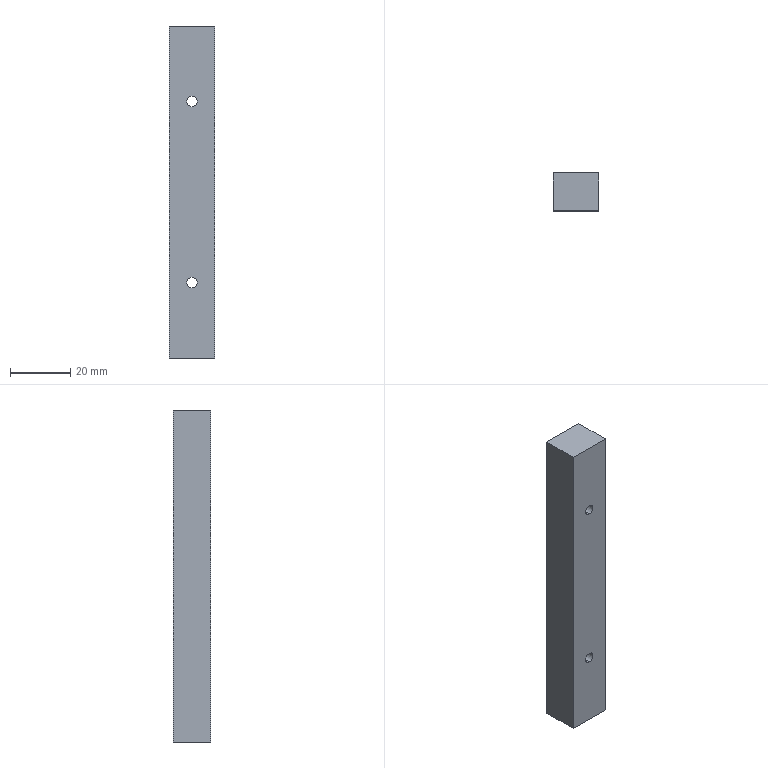Part | STEP file | Bag feed guide rail | 1 solid | 16 faces | box 15 x 12.5 x 110 mm | volume 20267 mm3 | cylinder 8 | plane 8 | commonest cylinder face diameters 3.4 x4 6 x4
STEP:
#1=CARTESIAN_POINT('',(0.,0.,0.));
#2=DIRECTION('',(0.,0.,1.));
#3=DIRECTION('',(1.,0.,0.));
#4=AXIS2_PLACEMENT_3D('',#1,#2,#3);
#5=CARTESIAN_POINT('',(0.,2.85,28.));
#6=VERTEX_POINT('',#5);
#7=CARTESIAN_POINT('',(0.,6.25,28.));
#8=VERTEX_POINT('',#7);
#9=CARTESIAN_POINT('',(0.,6.25,28.));
#10=DIRECTION('',(0.,1.,0.));
#11=VECTOR('',#10,1.);
#12=LINE('',#9,#11);
#13=CARTESIAN_POINT('',(0.,6.25,25.));
#14=DIRECTION('',(0.,1.,0.));
#15=DIRECTION('',(0.,0.,1.));
#16=AXIS2_PLACEMENT_3D('',#13,#14,#15);
#17=CYLINDRICAL_SURFACE('',#16,3.);
#18=CARTESIAN_POINT('',(6.283,0.));
#19=DIRECTION('',(0.,1.));
#20=VECTOR('',#19,1.);
#21=LINE('',#18,#20);
#22=(GEOMETRIC_REPRESENTATION_CONTEXT(2)PARAMETRIC_REPRESENTATION_CONTEXT()REPRESENTATION_CONTEXT('',''));
#23=DEFINITIONAL_REPRESENTATION('',(#21),#22);
#24=PCURVE('',#17,#23);
#25=CARTESIAN_POINT('',(0.,6.25,25.));
#26=DIRECTION('',(0.,1.,0.));
#27=DIRECTION('',(0.,0.,1.));
#28=AXIS2_PLACEMENT_3D('',#25,#26,#27);
#29=CYLINDRICAL_SURFACE('',#28,3.);
#30=CARTESIAN_POINT('',(0.,0.));
#31=DIRECTION('',(0.,1.));
#32=VECTOR('',#31,1.);
#33=LINE('',#30,#32);
#34=(GEOMETRIC_REPRESENTATION_CONTEXT(2)PARAMETRIC_REPRESENTATION_CONTEXT()REPRESENTATION_CONTEXT('',''));
#35=DEFINITIONAL_REPRESENTATION('',(#33),#34);
#36=PCURVE('',#29,#35);
#37=SURFACE_CURVE('',#12,(#24,#36),.PCURVE_S1.);
#38=EDGE_CURVE('',#6,#8,#37,.T.);
#39=ORIENTED_EDGE('',*,*,#38,.T.);
#40=CARTESIAN_POINT('',(0.,6.25,22.));
#41=VERTEX_POINT('',#40);
#42=CARTESIAN_POINT('',(0.,6.25,25.));
#43=DIRECTION('',(0.,1.,0.));
#44=DIRECTION('',(0.,0.,1.));
#45=AXIS2_PLACEMENT_3D('',#42,#43,#44);
#46=CIRCLE('',#45,3.);
#47=CARTESIAN_POINT('',(0.,0.));
#48=DIRECTION('',(1.,0.));
#49=VECTOR('',#48,1.);
#50=LINE('',#47,#49);
#51=(GEOMETRIC_REPRESENTATION_CONTEXT(2)PARAMETRIC_REPRESENTATION_CONTEXT()REPRESENTATION_CONTEXT('',''));
#52=DEFINITIONAL_REPRESENTATION('',(#50),#51);
#53=PCURVE('',#17,#52);
#54=CARTESIAN_POINT('',(-7.5,6.25,110.));
#55=DIRECTION('',(0.,-1.,0.));
#56=DIRECTION('',(0.,0.,-1.));
#57=AXIS2_PLACEMENT_3D('',#54,#55,#56);
#58=PLANE('',#57);
#59=CARTESIAN_POINT('',(82.,7.5));
#60=CARTESIAN_POINT('',(82.,12.696));
#61=CARTESIAN_POINT('',(86.5,10.098));
#62=CARTESIAN_POINT('',(91.,7.5));
#63=CARTESIAN_POINT('',(86.5,4.902));
#64=CARTESIAN_POINT('',(82.,2.304));
#65=CARTESIAN_POINT('',(82.,7.5));
#66=(BOUNDED_CURVE()B_SPLINE_CURVE(2,(#59,#60,#61,#62,#63,#64,#65),.UNSPECIFIED.,.T.,.F.)B_SPLINE_CURVE_WITH_KNOTS((1,2,2,2,2,1),(-2.094,0.,2.094,4.189,6.283,8.378),.UNSPECIFIED.)CURVE()GEOMETRIC_REPRESENTATION_ITEM()RATIONAL_B_SPLINE_CURVE((1.,0.5,1.,0.5,1.,0.5,1.))REPRESENTATION_ITEM(''));
#67=(GEOMETRIC_REPRESENTATION_CONTEXT(2)PARAMETRIC_REPRESENTATION_CONTEXT()REPRESENTATION_CONTEXT('',''));
#68=DEFINITIONAL_REPRESENTATION('',(#66),#67);
#69=PCURVE('',#58,#68);
#70=SURFACE_CURVE('',#46,(#53,#69),.PCURVE_S1.);
#71=EDGE_CURVE('',#41,#8,#70,.T.);
#72=ORIENTED_EDGE('',*,*,#71,.F.);
#73=CARTESIAN_POINT('',(0.,2.85,22.));
#74=VERTEX_POINT('',#73);
#75=CARTESIAN_POINT('',(0.,6.25,22.));
#76=DIRECTION('',(0.,1.,0.));
#77=VECTOR('',#76,1.);
#78=LINE('',#75,#77);
#79=CARTESIAN_POINT('',(3.142,0.));
#80=DIRECTION('',(0.,1.));
#81=VECTOR('',#80,1.);
#82=LINE('',#79,#81);
#83=(GEOMETRIC_REPRESENTATION_CONTEXT(2)PARAMETRIC_REPRESENTATION_CONTEXT()REPRESENTATION_CONTEXT('',''));
#84=DEFINITIONAL_REPRESENTATION('',(#82),#83);
#85=PCURVE('',#17,#84);
#86=CARTESIAN_POINT('',(3.142,0.));
#87=DIRECTION('',(0.,1.));
#88=VECTOR('',#87,1.);
#89=LINE('',#86,#88);
#90=(GEOMETRIC_REPRESENTATION_CONTEXT(2)PARAMETRIC_REPRESENTATION_CONTEXT()REPRESENTATION_CONTEXT('',''));
#91=DEFINITIONAL_REPRESENTATION('',(#89),#90);
#92=PCURVE('',#29,#91);
#93=SURFACE_CURVE('',#78,(#85,#92),.PCURVE_S1.);
#94=EDGE_CURVE('',#74,#41,#93,.T.);
#95=ORIENTED_EDGE('',*,*,#94,.F.);
#96=CARTESIAN_POINT('',(0.,2.85,25.));
#97=DIRECTION('',(0.,1.,0.));
#98=DIRECTION('',(0.,0.,1.));
#99=AXIS2_PLACEMENT_3D('',#96,#97,#98);
#100=CIRCLE('',#99,3.);
#101=CARTESIAN_POINT('',(0.,-3.4));
#102=DIRECTION('',(1.,0.));
#103=VECTOR('',#102,1.);
#104=LINE('',#101,#103);
#105=(GEOMETRIC_REPRESENTATION_CONTEXT(2)PARAMETRIC_REPRESENTATION_CONTEXT()REPRESENTATION_CONTEXT('',''));
#106=DEFINITIONAL_REPRESENTATION('',(#104),#105);
#107=PCURVE('',#17,#106);
#108=CARTESIAN_POINT('',(1.7,2.85,25.));
#109=DIRECTION('',(0.,-1.,0.));
#110=DIRECTION('',(0.,0.,-1.));
#111=AXIS2_PLACEMENT_3D('',#108,#109,#110);
#112=PLANE('',#111);
#113=CARTESIAN_POINT('',(-3.,-1.7));
#114=CARTESIAN_POINT('',(-3.,3.496));
#115=CARTESIAN_POINT('',(1.5,0.8981));
#116=CARTESIAN_POINT('',(6.,-1.7));
#117=CARTESIAN_POINT('',(1.5,-4.298));
#118=CARTESIAN_POINT('',(-3.,-6.896));
#119=CARTESIAN_POINT('',(-3.,-1.7));
#120=(BOUNDED_CURVE()B_SPLINE_CURVE(2,(#113,#114,#115,#116,#117,#118,#119),.UNSPECIFIED.,.T.,.F.)B_SPLINE_CURVE_WITH_KNOTS((1,2,2,2,2,1),(-2.094,0.,2.094,4.189,6.283,8.378),.UNSPECIFIED.)CURVE()GEOMETRIC_REPRESENTATION_ITEM()RATIONAL_B_SPLINE_CURVE((1.,0.5,1.,0.5,1.,0.5,1.))REPRESENTATION_ITEM(''));
#121=(GEOMETRIC_REPRESENTATION_CONTEXT(2)PARAMETRIC_REPRESENTATION_CONTEXT()REPRESENTATION_CONTEXT('',''));
#122=DEFINITIONAL_REPRESENTATION('',(#120),#121);
#123=PCURVE('',#112,#122);
#124=SURFACE_CURVE('',#100,(#107,#123),.PCURVE_S1.);
#125=EDGE_CURVE('',#74,#6,#124,.T.);
#126=ORIENTED_EDGE('',*,*,#125,.T.);
#127=EDGE_LOOP('',(#39,#72,#95,#126));
#128=FACE_BOUND('',#127,.F.);
#129=ADVANCED_FACE('',(#128),#17,.F.);
#130=CARTESIAN_POINT('',(0.,-6.25,26.7));
#131=VERTEX_POINT('',#130);
#132=CARTESIAN_POINT('',(0.,2.85,26.7));
#133=VERTEX_POINT('',#132);
#134=CARTESIAN_POINT('',(0.,6.25,26.7));
#135=DIRECTION('',(0.,1.,0.));
#136=VECTOR('',#135,1.);
#137=LINE('',#134,#136);
#138=CARTESIAN_POINT('',(0.,6.25,25.));
#139=DIRECTION('',(0.,1.,0.));
#140=DIRECTION('',(0.,0.,1.));
#141=AXIS2_PLACEMENT_3D('',#138,#139,#140);
#142=CYLINDRICAL_SURFACE('',#141,1.7);
#143=CARTESIAN_POINT('',(6.283,0.));
#144=DIRECTION('',(0.,1.));
#145=VECTOR('',#144,1.);
#146=LINE('',#143,#145);
#147=(GEOMETRIC_REPRESENTATION_CONTEXT(2)PARAMETRIC_REPRESENTATION_CONTEXT()REPRESENTATION_CONTEXT('',''));
#148=DEFINITIONAL_REPRESENTATION('',(#146),#147);
#149=PCURVE('',#142,#148);
#150=CARTESIAN_POINT('',(0.,6.25,25.));
#151=DIRECTION('',(0.,1.,0.));
#152=DIRECTION('',(0.,0.,1.));
#153=AXIS2_PLACEMENT_3D('',#150,#151,#152);
#154=CYLINDRICAL_SURFACE('',#153,1.7);
#155=CARTESIAN_POINT('',(0.,0.));
#156=DIRECTION('',(0.,1.));
#157=VECTOR('',#156,1.);
#158=LINE('',#155,#157);
#159=(GEOMETRIC_REPRESENTATION_CONTEXT(2)PARAMETRIC_REPRESENTATION_CONTEXT()REPRESENTATION_CONTEXT('',''));
#160=DEFINITIONAL_REPRESENTATION('',(#158),#159);
#161=PCURVE('',#154,#160);
#162=SURFACE_CURVE('',#137,(#149,#161),.PCURVE_S1.);
#163=EDGE_CURVE('',#131,#133,#162,.T.);
#164=ORIENTED_EDGE('',*,*,#163,.T.);
#165=CARTESIAN_POINT('',(0.,2.85,23.3));
#166=VERTEX_POINT('',#165);
#167=CARTESIAN_POINT('',(0.,2.85,25.));
#168=DIRECTION('',(0.,1.,0.));
#169=DIRECTION('',(0.,0.,1.));
#170=AXIS2_PLACEMENT_3D('',#167,#168,#169);
#171=CIRCLE('',#170,1.7);
#172=CARTESIAN_POINT('',(0.,-3.4));
#173=DIRECTION('',(1.,0.));
#174=VECTOR('',#173,1.);
#175=LINE('',#172,#174);
#176=(GEOMETRIC_REPRESENTATION_CONTEXT(2)PARAMETRIC_REPRESENTATION_CONTEXT()REPRESENTATION_CONTEXT('',''));
#177=DEFINITIONAL_REPRESENTATION('',(#175),#176);
#178=PCURVE('',#142,#177);
#179=CARTESIAN_POINT('',(-1.7,-1.7));
#180=CARTESIAN_POINT('',(-1.7,1.244));
#181=CARTESIAN_POINT('',(0.85,-0.2278));
#182=CARTESIAN_POINT('',(3.4,-1.7));
#183=CARTESIAN_POINT('',(0.85,-3.172));
#184=CARTESIAN_POINT('',(-1.7,-4.644));
#185=CARTESIAN_POINT('',(-1.7,-1.7));
#186=(BOUNDED_CURVE()B_SPLINE_CURVE(2,(#179,#180,#181,#182,#183,#184,#185),.UNSPECIFIED.,.T.,.F.)B_SPLINE_CURVE_WITH_KNOTS((1,2,2,2,2,1),(-2.094,0.,2.094,4.189,6.283,8.378),.UNSPECIFIED.)CURVE()GEOMETRIC_REPRESENTATION_ITEM()RATIONAL_B_SPLINE_CURVE((1.,0.5,1.,0.5,1.,0.5,1.))REPRESENTATION_ITEM(''));
#187=(GEOMETRIC_REPRESENTATION_CONTEXT(2)PARAMETRIC_REPRESENTATION_CONTEXT()REPRESENTATION_CONTEXT('',''));
#188=DEFINITIONAL_REPRESENTATION('',(#186),#187);
#189=PCURVE('',#112,#188);
#190=SURFACE_CURVE('',#171,(#178,#189),.PCURVE_S1.);
#191=EDGE_CURVE('',#166,#133,#190,.T.);
#192=ORIENTED_EDGE('',*,*,#191,.F.);
#193=CARTESIAN_POINT('',(0.,-6.25,23.3));
#194=VERTEX_POINT('',#193);
#195=CARTESIAN_POINT('',(0.,6.25,23.3));
#196=DIRECTION('',(0.,1.,0.));
#197=VECTOR('',#196,1.);
#198=LINE('',#195,#197);
#199=CARTESIAN_POINT('',(3.142,0.));
#200=DIRECTION('',(0.,1.));
#201=VECTOR('',#200,1.);
#202=LINE('',#199,#201);
#203=(GEOMETRIC_REPRESENTATION_CONTEXT(2)PARAMETRIC_REPRESENTATION_CONTEXT()REPRESENTATION_CONTEXT('',''));
#204=DEFINITIONAL_REPRESENTATION('',(#202),#203);
#205=PCURVE('',#142,#204);
#206=CARTESIAN_POINT('',(3.142,0.));
#207=DIRECTION('',(0.,1.));
#208=VECTOR('',#207,1.);
#209=LINE('',#206,#208);
#210=(GEOMETRIC_REPRESENTATION_CONTEXT(2)PARAMETRIC_REPRESENTATION_CONTEXT()REPRESENTATION_CONTEXT('',''));
#211=DEFINITIONAL_REPRESENTATION('',(#209),#210);
#212=PCURVE('',#154,#211);
#213=SURFACE_CURVE('',#198,(#205,#212),.PCURVE_S1.);
#214=EDGE_CURVE('',#194,#166,#213,.T.);
#215=ORIENTED_EDGE('',*,*,#214,.F.);
#216=CARTESIAN_POINT('',(0.,-6.25,25.));
#217=DIRECTION('',(0.,1.,0.));
#218=DIRECTION('',(0.,0.,1.));
#219=AXIS2_PLACEMENT_3D('',#216,#217,#218);
#220=CIRCLE('',#219,1.7);
#221=CARTESIAN_POINT('',(0.,-12.5));
#222=DIRECTION('',(1.,0.));
#223=VECTOR('',#222,1.);
#224=LINE('',#221,#223);
#225=(GEOMETRIC_REPRESENTATION_CONTEXT(2)PARAMETRIC_REPRESENTATION_CONTEXT()REPRESENTATION_CONTEXT('',''));
#226=DEFINITIONAL_REPRESENTATION('',(#224),#225);
#227=PCURVE('',#142,#226);
#228=CARTESIAN_POINT('',(-7.5,-6.25,110.));
#229=DIRECTION('',(0.,1.,0.));
#230=DIRECTION('',(0.,0.,1.));
#231=AXIS2_PLACEMENT_3D('',#228,#229,#230);
#232=PLANE('',#231);
#233=CARTESIAN_POINT('',(-85.,7.5));
#234=DIRECTION('',(1.,0.));
#235=AXIS2_PLACEMENT_2D('',#233,#234);
#236=CIRCLE('',#235,1.7);
#237=(GEOMETRIC_REPRESENTATION_CONTEXT(2)PARAMETRIC_REPRESENTATION_CONTEXT()REPRESENTATION_CONTEXT('',''));
#238=DEFINITIONAL_REPRESENTATION('',(#236),#237);
#239=PCURVE('',#232,#238);
#240=SURFACE_CURVE('',#220,(#227,#239),.PCURVE_S1.);
#241=EDGE_CURVE('',#194,#131,#240,.T.);
#242=ORIENTED_EDGE('',*,*,#241,.T.);
#243=EDGE_LOOP('',(#164,#192,#215,#242));
#244=FACE_BOUND('',#243,.F.);
#245=ADVANCED_FACE('',(#244),#142,.F.);
#246=CARTESIAN_POINT('',(0.,2.85,88.));
#247=VERTEX_POINT('',#246);
#248=CARTESIAN_POINT('',(0.,6.25,88.));
#249=VERTEX_POINT('',#248);
#250=CARTESIAN_POINT('',(0.,6.25,88.));
#251=DIRECTION('',(0.,1.,0.));
#252=VECTOR('',#251,1.);
#253=LINE('',#250,#252);
#254=CARTESIAN_POINT('',(0.,6.25,85.));
#255=DIRECTION('',(0.,1.,0.));
#256=DIRECTION('',(0.,0.,1.));
#257=AXIS2_PLACEMENT_3D('',#254,#255,#256);
#258=CYLINDRICAL_SURFACE('',#257,3.);
#259=CARTESIAN_POINT('',(6.283,0.));
#260=DIRECTION('',(0.,1.));
#261=VECTOR('',#260,1.);
#262=LINE('',#259,#261);
#263=(GEOMETRIC_REPRESENTATION_CONTEXT(2)PARAMETRIC_REPRESENTATION_CONTEXT()REPRESENTATION_CONTEXT('',''));
#264=DEFINITIONAL_REPRESENTATION('',(#262),#263);
#265=PCURVE('',#258,#264);
#266=CARTESIAN_POINT('',(0.,6.25,85.));
#267=DIRECTION('',(0.,1.,0.));
#268=DIRECTION('',(0.,0.,1.));
#269=AXIS2_PLACEMENT_3D('',#266,#267,#268);
#270=CYLINDRICAL_SURFACE('',#269,3.);
#271=CARTESIAN_POINT('',(0.,0.));
#272=DIRECTION('',(0.,1.));
#273=VECTOR('',#272,1.);
#274=LINE('',#271,#273);
#275=(GEOMETRIC_REPRESENTATION_CONTEXT(2)PARAMETRIC_REPRESENTATION_CONTEXT()REPRESENTATION_CONTEXT('',''));
#276=DEFINITIONAL_REPRESENTATION('',(#274),#275);
#277=PCURVE('',#270,#276);
#278=SURFACE_CURVE('',#253,(#265,#277),.PCURVE_S1.);
#279=EDGE_CURVE('',#247,#249,#278,.T.);
#280=ORIENTED_EDGE('',*,*,#279,.T.);
#281=CARTESIAN_POINT('',(0.,6.25,82.));
#282=VERTEX_POINT('',#281);
#283=CARTESIAN_POINT('',(0.,6.25,85.));
#284=DIRECTION('',(0.,1.,0.));
#285=DIRECTION('',(0.,0.,1.));
#286=AXIS2_PLACEMENT_3D('',#283,#284,#285);
#287=CIRCLE('',#286,3.);
#288=CARTESIAN_POINT('',(0.,0.));
#289=DIRECTION('',(1.,0.));
#290=VECTOR('',#289,1.);
#291=LINE('',#288,#290);
#292=(GEOMETRIC_REPRESENTATION_CONTEXT(2)PARAMETRIC_REPRESENTATION_CONTEXT()REPRESENTATION_CONTEXT('',''));
#293=DEFINITIONAL_REPRESENTATION('',(#291),#292);
#294=PCURVE('',#258,#293);
#295=CARTESIAN_POINT('',(22.,7.5));
#296=CARTESIAN_POINT('',(22.,12.696));
#297=CARTESIAN_POINT('',(26.5,10.098));
#298=CARTESIAN_POINT('',(31.,7.5));
#299=CARTESIAN_POINT('',(26.5,4.902));
#300=CARTESIAN_POINT('',(22.,2.304));
#301=CARTESIAN_POINT('',(22.,7.5));
#302=(BOUNDED_CURVE()B_SPLINE_CURVE(2,(#295,#296,#297,#298,#299,#300,#301),.UNSPECIFIED.,.T.,.F.)B_SPLINE_CURVE_WITH_KNOTS((1,2,2,2,2,1),(-2.094,0.,2.094,4.189,6.283,8.378),.UNSPECIFIED.)CURVE()GEOMETRIC_REPRESENTATION_ITEM()RATIONAL_B_SPLINE_CURVE((1.,0.5,1.,0.5,1.,0.5,1.))REPRESENTATION_ITEM(''));
#303=(GEOMETRIC_REPRESENTATION_CONTEXT(2)PARAMETRIC_REPRESENTATION_CONTEXT()REPRESENTATION_CONTEXT('',''));
#304=DEFINITIONAL_REPRESENTATION('',(#302),#303);
#305=PCURVE('',#58,#304);
#306=SURFACE_CURVE('',#287,(#294,#305),.PCURVE_S1.);
#307=EDGE_CURVE('',#282,#249,#306,.T.);
#308=ORIENTED_EDGE('',*,*,#307,.F.);
#309=CARTESIAN_POINT('',(0.,2.85,82.));
#310=VERTEX_POINT('',#309);
#311=CARTESIAN_POINT('',(0.,6.25,82.));
#312=DIRECTION('',(0.,1.,0.));
#313=VECTOR('',#312,1.);
#314=LINE('',#311,#313);
#315=CARTESIAN_POINT('',(3.142,0.));
#316=DIRECTION('',(0.,1.));
#317=VECTOR('',#316,1.);
#318=LINE('',#315,#317);
#319=(GEOMETRIC_REPRESENTATION_CONTEXT(2)PARAMETRIC_REPRESENTATION_CONTEXT()REPRESENTATION_CONTEXT('',''));
#320=DEFINITIONAL_REPRESENTATION('',(#318),#319);
#321=PCURVE('',#258,#320);
#322=CARTESIAN_POINT('',(3.142,0.));
#323=DIRECTION('',(0.,1.));
#324=VECTOR('',#323,1.);
#325=LINE('',#322,#324);
#326=(GEOMETRIC_REPRESENTATION_CONTEXT(2)PARAMETRIC_REPRESENTATION_CONTEXT()REPRESENTATION_CONTEXT('',''));
#327=DEFINITIONAL_REPRESENTATION('',(#325),#326);
#328=PCURVE('',#270,#327);
#329=SURFACE_CURVE('',#314,(#321,#328),.PCURVE_S1.);
#330=EDGE_CURVE('',#310,#282,#329,.T.);
#331=ORIENTED_EDGE('',*,*,#330,.F.);
#332=CARTESIAN_POINT('',(0.,2.85,85.));
#333=DIRECTION('',(0.,1.,0.));
#334=DIRECTION('',(0.,0.,1.));
#335=AXIS2_PLACEMENT_3D('',#332,#333,#334);
#336=CIRCLE('',#335,3.);
#337=CARTESIAN_POINT('',(0.,-3.4));
#338=DIRECTION('',(1.,0.));
#339=VECTOR('',#338,1.);
#340=LINE('',#337,#339);
#341=(GEOMETRIC_REPRESENTATION_CONTEXT(2)PARAMETRIC_REPRESENTATION_CONTEXT()REPRESENTATION_CONTEXT('',''));
#342=DEFINITIONAL_REPRESENTATION('',(#340),#341);
#343=PCURVE('',#258,#342);
#344=CARTESIAN_POINT('',(1.7,2.85,85.));
#345=DIRECTION('',(0.,-1.,0.));
#346=DIRECTION('',(0.,0.,-1.));
#347=AXIS2_PLACEMENT_3D('',#344,#345,#346);
#348=PLANE('',#347);
#349=CARTESIAN_POINT('',(-3.,-1.7));
#350=CARTESIAN_POINT('',(-3.,3.496));
#351=CARTESIAN_POINT('',(1.5,0.8981));
#352=CARTESIAN_POINT('',(6.,-1.7));
#353=CARTESIAN_POINT('',(1.5,-4.298));
#354=CARTESIAN_POINT('',(-3.,-6.896));
#355=CARTESIAN_POINT('',(-3.,-1.7));
#356=(BOUNDED_CURVE()B_SPLINE_CURVE(2,(#349,#350,#351,#352,#353,#354,#355),.UNSPECIFIED.,.T.,.F.)B_SPLINE_CURVE_WITH_KNOTS((1,2,2,2,2,1),(-2.094,0.,2.094,4.189,6.283,8.378),.UNSPECIFIED.)CURVE()GEOMETRIC_REPRESENTATION_ITEM()RATIONAL_B_SPLINE_CURVE((1.,0.5,1.,0.5,1.,0.5,1.))REPRESENTATION_ITEM(''));
#357=(GEOMETRIC_REPRESENTATION_CONTEXT(2)PARAMETRIC_REPRESENTATION_CONTEXT()REPRESENTATION_CONTEXT('',''));
#358=DEFINITIONAL_REPRESENTATION('',(#356),#357);
#359=PCURVE('',#348,#358);
#360=SURFACE_CURVE('',#336,(#343,#359),.PCURVE_S1.);
#361=EDGE_CURVE('',#310,#247,#360,.T.);
#362=ORIENTED_EDGE('',*,*,#361,.T.);
#363=EDGE_LOOP('',(#280,#308,#331,#362));
#364=FACE_BOUND('',#363,.F.);
#365=ADVANCED_FACE('',(#364),#258,.F.);
#366=CARTESIAN_POINT('',(0.,-6.25,86.7));
#367=VERTEX_POINT('',#366);
#368=CARTESIAN_POINT('',(0.,2.85,86.7));
#369=VERTEX_POINT('',#368);
#370=CARTESIAN_POINT('',(0.,6.25,86.7));
#371=DIRECTION('',(0.,1.,0.));
#372=VECTOR('',#371,1.);
#373=LINE('',#370,#372);
#374=CARTESIAN_POINT('',(0.,6.25,85.));
#375=DIRECTION('',(0.,1.,0.));
#376=DIRECTION('',(0.,0.,1.));
#377=AXIS2_PLACEMENT_3D('',#374,#375,#376);
#378=CYLINDRICAL_SURFACE('',#377,1.7);
#379=CARTESIAN_POINT('',(6.283,0.));
#380=DIRECTION('',(0.,1.));
#381=VECTOR('',#380,1.);
#382=LINE('',#379,#381);
#383=(GEOMETRIC_REPRESENTATION_CONTEXT(2)PARAMETRIC_REPRESENTATION_CONTEXT()REPRESENTATION_CONTEXT('',''));
#384=DEFINITIONAL_REPRESENTATION('',(#382),#383);
#385=PCURVE('',#378,#384);
#386=CARTESIAN_POINT('',(0.,6.25,85.));
#387=DIRECTION('',(0.,1.,0.));
#388=DIRECTION('',(0.,0.,1.));
#389=AXIS2_PLACEMENT_3D('',#386,#387,#388);
#390=CYLINDRICAL_SURFACE('',#389,1.7);
#391=CARTESIAN_POINT('',(0.,0.));
#392=DIRECTION('',(0.,1.));
#393=VECTOR('',#392,1.);
#394=LINE('',#391,#393);
#395=(GEOMETRIC_REPRESENTATION_CONTEXT(2)PARAMETRIC_REPRESENTATION_CONTEXT()REPRESENTATION_CONTEXT('',''));
#396=DEFINITIONAL_REPRESENTATION('',(#394),#395);
#397=PCURVE('',#390,#396);
#398=SURFACE_CURVE('',#373,(#385,#397),.PCURVE_S1.);
#399=EDGE_CURVE('',#367,#369,#398,.T.);
#400=ORIENTED_EDGE('',*,*,#399,.T.);
#401=CARTESIAN_POINT('',(0.,2.85,83.3));
#402=VERTEX_POINT('',#401);
#403=CARTESIAN_POINT('',(0.,2.85,85.));
#404=DIRECTION('',(0.,1.,0.));
#405=DIRECTION('',(0.,0.,1.));
#406=AXIS2_PLACEMENT_3D('',#403,#404,#405);
#407=CIRCLE('',#406,1.7);
#408=CARTESIAN_POINT('',(0.,-3.4));
#409=DIRECTION('',(1.,0.));
#410=VECTOR('',#409,1.);
#411=LINE('',#408,#410);
#412=(GEOMETRIC_REPRESENTATION_CONTEXT(2)PARAMETRIC_REPRESENTATION_CONTEXT()REPRESENTATION_CONTEXT('',''));
#413=DEFINITIONAL_REPRESENTATION('',(#411),#412);
#414=PCURVE('',#378,#413);
#415=CARTESIAN_POINT('',(-1.7,-1.7));
#416=CARTESIAN_POINT('',(-1.7,1.244));
#417=CARTESIAN_POINT('',(0.85,-0.2278));
#418=CARTESIAN_POINT('',(3.4,-1.7));
#419=CARTESIAN_POINT('',(0.85,-3.172));
#420=CARTESIAN_POINT('',(-1.7,-4.644));
#421=CARTESIAN_POINT('',(-1.7,-1.7));
#422=(BOUNDED_CURVE()B_SPLINE_CURVE(2,(#415,#416,#417,#418,#419,#420,#421),.UNSPECIFIED.,.T.,.F.)B_SPLINE_CURVE_WITH_KNOTS((1,2,2,2,2,1),(-2.094,0.,2.094,4.189,6.283,8.378),.UNSPECIFIED.)CURVE()GEOMETRIC_REPRESENTATION_ITEM()RATIONAL_B_SPLINE_CURVE((1.,0.5,1.,0.5,1.,0.5,1.))REPRESENTATION_ITEM(''));
#423=(GEOMETRIC_REPRESENTATION_CONTEXT(2)PARAMETRIC_REPRESENTATION_CONTEXT()REPRESENTATION_CONTEXT('',''));
#424=DEFINITIONAL_REPRESENTATION('',(#422),#423);
#425=PCURVE('',#348,#424);
#426=SURFACE_CURVE('',#407,(#414,#425),.PCURVE_S1.);
#427=EDGE_CURVE('',#402,#369,#426,.T.);
#428=ORIENTED_EDGE('',*,*,#427,.F.);
#429=CARTESIAN_POINT('',(0.,-6.25,83.3));
#430=VERTEX_POINT('',#429);
#431=CARTESIAN_POINT('',(0.,6.25,83.3));
#432=DIRECTION('',(0.,1.,0.));
#433=VECTOR('',#432,1.);
#434=LINE('',#431,#433);
#435=CARTESIAN_POINT('',(3.142,0.));
#436=DIRECTION('',(0.,1.));
#437=VECTOR('',#436,1.);
#438=LINE('',#435,#437);
#439=(GEOMETRIC_REPRESENTATION_CONTEXT(2)PARAMETRIC_REPRESENTATION_CONTEXT()REPRESENTATION_CONTEXT('',''));
#440=DEFINITIONAL_REPRESENTATION('',(#438),#439);
#441=PCURVE('',#378,#440);
#442=CARTESIAN_POINT('',(3.142,0.));
#443=DIRECTION('',(0.,1.));
#444=VECTOR('',#443,1.);
#445=LINE('',#442,#444);
#446=(GEOMETRIC_REPRESENTATION_CONTEXT(2)PARAMETRIC_REPRESENTATION_CONTEXT()REPRESENTATION_CONTEXT('',''));
#447=DEFINITIONAL_REPRESENTATION('',(#445),#446);
#448=PCURVE('',#390,#447);
#449=SURFACE_CURVE('',#434,(#441,#448),.PCURVE_S1.);
#450=EDGE_CURVE('',#430,#402,#449,.T.);
#451=ORIENTED_EDGE('',*,*,#450,.F.);
#452=CARTESIAN_POINT('',(0.,-6.25,85.));
#453=DIRECTION('',(0.,1.,0.));
#454=DIRECTION('',(0.,0.,1.));
#455=AXIS2_PLACEMENT_3D('',#452,#453,#454);
#456=CIRCLE('',#455,1.7);
#457=CARTESIAN_POINT('',(0.,-12.5));
#458=DIRECTION('',(1.,0.));
#459=VECTOR('',#458,1.);
#460=LINE('',#457,#459);
#461=(GEOMETRIC_REPRESENTATION_CONTEXT(2)PARAMETRIC_REPRESENTATION_CONTEXT()REPRESENTATION_CONTEXT('',''));
#462=DEFINITIONAL_REPRESENTATION('',(#460),#461);
#463=PCURVE('',#378,#462);
#464=CARTESIAN_POINT('',(-25.,7.5));
#465=DIRECTION('',(1.,0.));
#466=AXIS2_PLACEMENT_2D('',#464,#465);
#467=CIRCLE('',#466,1.7);
#468=(GEOMETRIC_REPRESENTATION_CONTEXT(2)PARAMETRIC_REPRESENTATION_CONTEXT()REPRESENTATION_CONTEXT('',''));
#469=DEFINITIONAL_REPRESENTATION('',(#467),#468);
#470=PCURVE('',#232,#469);
#471=SURFACE_CURVE('',#456,(#463,#470),.PCURVE_S1.);
#472=EDGE_CURVE('',#430,#367,#471,.T.);
#473=ORIENTED_EDGE('',*,*,#472,.T.);
#474=EDGE_LOOP('',(#400,#428,#451,#473));
#475=FACE_BOUND('',#474,.F.);
#476=ADVANCED_FACE('',(#475),#378,.F.);
#477=CARTESIAN_POINT('',(7.5,-6.25,0.));
#478=VERTEX_POINT('',#477);
#479=CARTESIAN_POINT('',(7.5,6.25,0.));
#480=VERTEX_POINT('',#479);
#481=CARTESIAN_POINT('',(7.5,-6.25,0.));
#482=DIRECTION('',(0.,1.,0.));
#483=VECTOR('',#482,1.);
#484=LINE('',#481,#483);
#485=CARTESIAN_POINT('',(7.5,-6.25,110.));
#486=DIRECTION('',(-1.,0.,0.));
#487=DIRECTION('',(0.,0.,1.));
#488=AXIS2_PLACEMENT_3D('',#485,#486,#487);
#489=PLANE('',#488);
#490=CARTESIAN_POINT('',(-110.,0.));
#491=DIRECTION('',(0.,1.));
#492=VECTOR('',#491,1.);
#493=LINE('',#490,#492);
#494=(GEOMETRIC_REPRESENTATION_CONTEXT(2)PARAMETRIC_REPRESENTATION_CONTEXT()REPRESENTATION_CONTEXT('',''));
#495=DEFINITIONAL_REPRESENTATION('',(#493),#494);
#496=PCURVE('',#489,#495);
#497=CARTESIAN_POINT('',(0.,0.,0.));
#498=DIRECTION('',(0.,0.,-1.));
#499=DIRECTION('',(-1.,0.,0.));
#500=AXIS2_PLACEMENT_3D('',#497,#498,#499);
#501=PLANE('',#500);
#502=CARTESIAN_POINT('',(-7.5,-6.25));
#503=DIRECTION('',(0.,1.));
#504=VECTOR('',#503,1.);
#505=LINE('',#502,#504);
#506=(GEOMETRIC_REPRESENTATION_CONTEXT(2)PARAMETRIC_REPRESENTATION_CONTEXT()REPRESENTATION_CONTEXT('',''));
#507=DEFINITIONAL_REPRESENTATION('',(#505),#506);
#508=PCURVE('',#501,#507);
#509=SURFACE_CURVE('',#484,(#496,#508),.PCURVE_S1.);
#510=EDGE_CURVE('',#478,#480,#509,.T.);
#511=ORIENTED_EDGE('',*,*,#510,.T.);
#512=CARTESIAN_POINT('',(7.5,6.25,110.));
#513=VERTEX_POINT('',#512);
#514=CARTESIAN_POINT('',(7.5,6.25,110.));
#515=DIRECTION('',(0.,0.,-1.));
#516=VECTOR('',#515,1.);
#517=LINE('',#514,#516);
#518=CARTESIAN_POINT('',(0.,12.5));
#519=DIRECTION('',(-1.,0.));
#520=VECTOR('',#519,1.);
#521=LINE('',#518,#520);
#522=(GEOMETRIC_REPRESENTATION_CONTEXT(2)PARAMETRIC_REPRESENTATION_CONTEXT()REPRESENTATION_CONTEXT('',''));
#523=DEFINITIONAL_REPRESENTATION('',(#521),#522);
#524=PCURVE('',#489,#523);
#525=CARTESIAN_POINT('',(0.,15.));
#526=DIRECTION('',(1.,0.));
#527=VECTOR('',#526,1.);
#528=LINE('',#525,#527);
#529=(GEOMETRIC_REPRESENTATION_CONTEXT(2)PARAMETRIC_REPRESENTATION_CONTEXT()REPRESENTATION_CONTEXT('',''));
#530=DEFINITIONAL_REPRESENTATION('',(#528),#529);
#531=PCURVE('',#58,#530);
#532=SURFACE_CURVE('',#517,(#524,#531),.PCURVE_S1.);
#533=EDGE_CURVE('',#513,#480,#532,.T.);
#534=ORIENTED_EDGE('',*,*,#533,.F.);
#535=CARTESIAN_POINT('',(7.5,-6.25,110.));
#536=VERTEX_POINT('',#535);
#537=CARTESIAN_POINT('',(7.5,-6.25,110.));
#538=DIRECTION('',(0.,1.,0.));
#539=VECTOR('',#538,1.);
#540=LINE('',#537,#539);
#541=CARTESIAN_POINT('',(0.,0.));
#542=DIRECTION('',(0.,1.));
#543=VECTOR('',#542,1.);
#544=LINE('',#541,#543);
#545=(GEOMETRIC_REPRESENTATION_CONTEXT(2)PARAMETRIC_REPRESENTATION_CONTEXT()REPRESENTATION_CONTEXT('',''));
#546=DEFINITIONAL_REPRESENTATION('',(#544),#545);
#547=PCURVE('',#489,#546);
#548=CARTESIAN_POINT('',(0.,0.,110.));
#549=DIRECTION('',(0.,0.,-1.));
#550=DIRECTION('',(-1.,0.,0.));
#551=AXIS2_PLACEMENT_3D('',#548,#549,#550);
#552=PLANE('',#551);
#553=CARTESIAN_POINT('',(-7.5,-6.25));
#554=DIRECTION('',(0.,1.));
#555=VECTOR('',#554,1.);
#556=LINE('',#553,#555);
#557=(GEOMETRIC_REPRESENTATION_CONTEXT(2)PARAMETRIC_REPRESENTATION_CONTEXT()REPRESENTATION_CONTEXT('',''));
#558=DEFINITIONAL_REPRESENTATION('',(#556),#557);
#559=PCURVE('',#552,#558);
#560=SURFACE_CURVE('',#540,(#547,#559),.PCURVE_S1.);
#561=EDGE_CURVE('',#536,#513,#560,.T.);
#562=ORIENTED_EDGE('',*,*,#561,.F.);
#563=CARTESIAN_POINT('',(7.5,-6.25,110.));
#564=DIRECTION('',(0.,0.,-1.));
#565=VECTOR('',#564,1.);
#566=LINE('',#563,#565);
#567=CARTESIAN_POINT('',(0.,0.));
#568=DIRECTION('',(-1.,0.));
#569=VECTOR('',#568,1.);
#570=LINE('',#567,#569);
#571=(GEOMETRIC_REPRESENTATION_CONTEXT(2)PARAMETRIC_REPRESENTATION_CONTEXT()REPRESENTATION_CONTEXT('',''));
#572=DEFINITIONAL_REPRESENTATION('',(#570),#571);
#573=PCURVE('',#489,#572);
#574=CARTESIAN_POINT('',(0.,15.));
#575=DIRECTION('',(-1.,0.));
#576=VECTOR('',#575,1.);
#577=LINE('',#574,#576);
#578=(GEOMETRIC_REPRESENTATION_CONTEXT(2)PARAMETRIC_REPRESENTATION_CONTEXT()REPRESENTATION_CONTEXT('',''));
#579=DEFINITIONAL_REPRESENTATION('',(#577),#578);
#580=PCURVE('',#232,#579);
#581=SURFACE_CURVE('',#566,(#573,#580),.PCURVE_S1.);
#582=EDGE_CURVE('',#536,#478,#581,.T.);
#583=ORIENTED_EDGE('',*,*,#582,.T.);
#584=EDGE_LOOP('',(#511,#534,#562,#583));
#585=FACE_BOUND('',#584,.T.);
#586=ADVANCED_FACE('',(#585),#489,.F.);
#587=CARTESIAN_POINT('',(0.,6.25,25.));
#588=DIRECTION('',(0.,1.,0.));
#589=DIRECTION('',(0.,0.,1.));
#590=AXIS2_PLACEMENT_3D('',#587,#588,#589);
#591=CIRCLE('',#590,3.);
#592=CARTESIAN_POINT('',(82.,7.5));
#593=CARTESIAN_POINT('',(82.,12.696));
#594=CARTESIAN_POINT('',(86.5,10.098));
#595=CARTESIAN_POINT('',(91.,7.5));
#596=CARTESIAN_POINT('',(86.5,4.902));
#597=CARTESIAN_POINT('',(82.,2.304));
#598=CARTESIAN_POINT('',(82.,7.5));
#599=(BOUNDED_CURVE()B_SPLINE_CURVE(2,(#592,#593,#594,#595,#596,#597,#598),.UNSPECIFIED.,.T.,.F.)B_SPLINE_CURVE_WITH_KNOTS((1,2,2,2,2,1),(-2.094,0.,2.094,4.189,6.283,8.378),.UNSPECIFIED.)CURVE()GEOMETRIC_REPRESENTATION_ITEM()RATIONAL_B_SPLINE_CURVE((1.,0.5,1.,0.5,1.,0.5,1.))REPRESENTATION_ITEM(''));
#600=(GEOMETRIC_REPRESENTATION_CONTEXT(2)PARAMETRIC_REPRESENTATION_CONTEXT()REPRESENTATION_CONTEXT('',''));
#601=DEFINITIONAL_REPRESENTATION('',(#599),#600);
#602=PCURVE('',#58,#601);
#603=CARTESIAN_POINT('',(0.,0.));
#604=DIRECTION('',(1.,0.));
#605=VECTOR('',#604,1.);
#606=LINE('',#603,#605);
#607=(GEOMETRIC_REPRESENTATION_CONTEXT(2)PARAMETRIC_REPRESENTATION_CONTEXT()REPRESENTATION_CONTEXT('',''));
#608=DEFINITIONAL_REPRESENTATION('',(#606),#607);
#609=PCURVE('',#29,#608);
#610=SURFACE_CURVE('',#591,(#602,#609),.PCURVE_S1.);
#611=EDGE_CURVE('',#8,#41,#610,.T.);
#612=ORIENTED_EDGE('',*,*,#611,.F.);
#613=ORIENTED_EDGE('',*,*,#71,.F.);
#614=EDGE_LOOP('',(#612,#613));
#615=FACE_BOUND('',#614,.T.);
#616=CARTESIAN_POINT('',(0.,6.25,85.));
#617=DIRECTION('',(0.,1.,0.));
#618=DIRECTION('',(0.,0.,1.));
#619=AXIS2_PLACEMENT_3D('',#616,#617,#618);
#620=CIRCLE('',#619,3.);
#621=CARTESIAN_POINT('',(22.,7.5));
#622=CARTESIAN_POINT('',(22.,12.696));
#623=CARTESIAN_POINT('',(26.5,10.098));
#624=CARTESIAN_POINT('',(31.,7.5));
#625=CARTESIAN_POINT('',(26.5,4.902));
#626=CARTESIAN_POINT('',(22.,2.304));
#627=CARTESIAN_POINT('',(22.,7.5));
#628=(BOUNDED_CURVE()B_SPLINE_CURVE(2,(#621,#622,#623,#624,#625,#626,#627),.UNSPECIFIED.,.T.,.F.)B_SPLINE_CURVE_WITH_KNOTS((1,2,2,2,2,1),(-2.094,0.,2.094,4.189,6.283,8.378),.UNSPECIFIED.)CURVE()GEOMETRIC_REPRESENTATION_ITEM()RATIONAL_B_SPLINE_CURVE((1.,0.5,1.,0.5,1.,0.5,1.))REPRESENTATION_ITEM(''));
#629=(GEOMETRIC_REPRESENTATION_CONTEXT(2)PARAMETRIC_REPRESENTATION_CONTEXT()REPRESENTATION_CONTEXT('',''));
#630=DEFINITIONAL_REPRESENTATION('',(#628),#629);
#631=PCURVE('',#58,#630);
#632=CARTESIAN_POINT('',(0.,0.));
#633=DIRECTION('',(1.,0.));
#634=VECTOR('',#633,1.);
#635=LINE('',#632,#634);
#636=(GEOMETRIC_REPRESENTATION_CONTEXT(2)PARAMETRIC_REPRESENTATION_CONTEXT()REPRESENTATION_CONTEXT('',''));
#637=DEFINITIONAL_REPRESENTATION('',(#635),#636);
#638=PCURVE('',#270,#637);
#639=SURFACE_CURVE('',#620,(#631,#638),.PCURVE_S1.);
#640=EDGE_CURVE('',#249,#282,#639,.T.);
#641=ORIENTED_EDGE('',*,*,#640,.F.);
#642=ORIENTED_EDGE('',*,*,#307,.F.);
#643=EDGE_LOOP('',(#641,#642));
#644=FACE_BOUND('',#643,.T.);
#645=CARTESIAN_POINT('',(-7.5,6.25,0.));
#646=VERTEX_POINT('',#645);
#647=CARTESIAN_POINT('',(-7.5,6.25,0.));
#648=DIRECTION('',(-1.,0.,0.));
#649=VECTOR('',#648,1.);
#650=LINE('',#647,#649);
#651=CARTESIAN_POINT('',(110.,0.));
#652=DIRECTION('',(0.,-1.));
#653=VECTOR('',#652,1.);
#654=LINE('',#651,#653);
#655=(GEOMETRIC_REPRESENTATION_CONTEXT(2)PARAMETRIC_REPRESENTATION_CONTEXT()REPRESENTATION_CONTEXT('',''));
#656=DEFINITIONAL_REPRESENTATION('',(#654),#655);
#657=PCURVE('',#58,#656);
#658=CARTESIAN_POINT('',(7.5,6.25));
#659=DIRECTION('',(1.,0.));
#660=VECTOR('',#659,1.);
#661=LINE('',#658,#660);
#662=(GEOMETRIC_REPRESENTATION_CONTEXT(2)PARAMETRIC_REPRESENTATION_CONTEXT()REPRESENTATION_CONTEXT('',''));
#663=DEFINITIONAL_REPRESENTATION('',(#661),#662);
#664=PCURVE('',#501,#663);
#665=SURFACE_CURVE('',#650,(#657,#664),.PCURVE_S1.);
#666=EDGE_CURVE('',#480,#646,#665,.T.);
#667=ORIENTED_EDGE('',*,*,#666,.T.);
#668=CARTESIAN_POINT('',(-7.5,6.25,110.));
#669=VERTEX_POINT('',#668);
#670=CARTESIAN_POINT('',(-7.5,6.25,110.));
#671=DIRECTION('',(0.,0.,-1.));
#672=VECTOR('',#671,1.);
#673=LINE('',#670,#672);
#674=CARTESIAN_POINT('',(0.,0.));
#675=DIRECTION('',(1.,0.));
#676=VECTOR('',#675,1.);
#677=LINE('',#674,#676);
#678=(GEOMETRIC_REPRESENTATION_CONTEXT(2)PARAMETRIC_REPRESENTATION_CONTEXT()REPRESENTATION_CONTEXT('',''));
#679=DEFINITIONAL_REPRESENTATION('',(#677),#678);
#680=PCURVE('',#58,#679);
#681=CARTESIAN_POINT('',(-7.5,-6.25,110.));
#682=DIRECTION('',(1.,0.,0.));
#683=DIRECTION('',(0.,0.,-1.));
#684=AXIS2_PLACEMENT_3D('',#681,#682,#683);
#685=PLANE('',#684);
#686=CARTESIAN_POINT('',(0.,12.5));
#687=DIRECTION('',(1.,0.));
#688=VECTOR('',#687,1.);
#689=LINE('',#686,#688);
#690=(GEOMETRIC_REPRESENTATION_CONTEXT(2)PARAMETRIC_REPRESENTATION_CONTEXT()REPRESENTATION_CONTEXT('',''));
#691=DEFINITIONAL_REPRESENTATION('',(#689),#690);
#692=PCURVE('',#685,#691);
#693=SURFACE_CURVE('',#673,(#680,#692),.PCURVE_S1.);
#694=EDGE_CURVE('',#669,#646,#693,.T.);
#695=ORIENTED_EDGE('',*,*,#694,.F.);
#696=CARTESIAN_POINT('',(-7.5,6.25,110.));
#697=DIRECTION('',(-1.,0.,0.));
#698=VECTOR('',#697,1.);
#699=LINE('',#696,#698);
#700=CARTESIAN_POINT('',(0.,0.));
#701=DIRECTION('',(0.,-1.));
#702=VECTOR('',#701,1.);
#703=LINE('',#700,#702);
#704=(GEOMETRIC_REPRESENTATION_CONTEXT(2)PARAMETRIC_REPRESENTATION_CONTEXT()REPRESENTATION_CONTEXT('',''));
#705=DEFINITIONAL_REPRESENTATION('',(#703),#704);
#706=PCURVE('',#58,#705);
#707=CARTESIAN_POINT('',(7.5,6.25));
#708=DIRECTION('',(1.,0.));
#709=VECTOR('',#708,1.);
#710=LINE('',#707,#709);
#711=(GEOMETRIC_REPRESENTATION_CONTEXT(2)PARAMETRIC_REPRESENTATION_CONTEXT()REPRESENTATION_CONTEXT('',''));
#712=DEFINITIONAL_REPRESENTATION('',(#710),#711);
#713=PCURVE('',#552,#712);
#714=SURFACE_CURVE('',#699,(#706,#713),.PCURVE_S1.);
#715=EDGE_CURVE('',#513,#669,#714,.T.);
#716=ORIENTED_EDGE('',*,*,#715,.F.);
#717=ORIENTED_EDGE('',*,*,#533,.T.);
#718=EDGE_LOOP('',(#667,#695,#716,#717));
#719=FACE_BOUND('',#718,.T.);
#720=ADVANCED_FACE('',(#615,#644,#719),#58,.F.);
#721=CARTESIAN_POINT('',(-7.5,-6.25,0.));
#722=VERTEX_POINT('',#721);
#723=CARTESIAN_POINT('',(-7.5,-6.25,0.));
#724=DIRECTION('',(0.,-1.,0.));
#725=VECTOR('',#724,1.);
#726=LINE('',#723,#725);
#727=CARTESIAN_POINT('',(110.,0.));
#728=DIRECTION('',(0.,-1.));
#729=VECTOR('',#728,1.);
#730=LINE('',#727,#729);
#731=(GEOMETRIC_REPRESENTATION_CONTEXT(2)PARAMETRIC_REPRESENTATION_CONTEXT()REPRESENTATION_CONTEXT('',''));
#732=DEFINITIONAL_REPRESENTATION('',(#730),#731);
#733=PCURVE('',#685,#732);
#734=CARTESIAN_POINT('',(7.5,-6.25));
#735=DIRECTION('',(0.,-1.));
#736=VECTOR('',#735,1.);
#737=LINE('',#734,#736);
#738=(GEOMETRIC_REPRESENTATION_CONTEXT(2)PARAMETRIC_REPRESENTATION_CONTEXT()REPRESENTATION_CONTEXT('',''));
#739=DEFINITIONAL_REPRESENTATION('',(#737),#738);
#740=PCURVE('',#501,#739);
#741=SURFACE_CURVE('',#726,(#733,#740),.PCURVE_S1.);
#742=EDGE_CURVE('',#646,#722,#741,.T.);
#743=ORIENTED_EDGE('',*,*,#742,.T.);
#744=CARTESIAN_POINT('',(-7.5,-6.25,110.));
#745=VERTEX_POINT('',#744);
#746=CARTESIAN_POINT('',(-7.5,-6.25,110.));
#747=DIRECTION('',(0.,0.,-1.));
#748=VECTOR('',#747,1.);
#749=LINE('',#746,#748);
#750=CARTESIAN_POINT('',(0.,0.));
#751=DIRECTION('',(1.,0.));
#752=VECTOR('',#751,1.);
#753=LINE('',#750,#752);
#754=(GEOMETRIC_REPRESENTATION_CONTEXT(2)PARAMETRIC_REPRESENTATION_CONTEXT()REPRESENTATION_CONTEXT('',''));
#755=DEFINITIONAL_REPRESENTATION('',(#753),#754);
#756=PCURVE('',#685,#755);
#757=CARTESIAN_POINT('',(0.,0.));
#758=DIRECTION('',(-1.,0.));
#759=VECTOR('',#758,1.);
#760=LINE('',#757,#759);
#761=(GEOMETRIC_REPRESENTATION_CONTEXT(2)PARAMETRIC_REPRESENTATION_CONTEXT()REPRESENTATION_CONTEXT('',''));
#762=DEFINITIONAL_REPRESENTATION('',(#760),#761);
#763=PCURVE('',#232,#762);
#764=SURFACE_CURVE('',#749,(#756,#763),.PCURVE_S1.);
#765=EDGE_CURVE('',#745,#722,#764,.T.);
#766=ORIENTED_EDGE('',*,*,#765,.F.);
#767=CARTESIAN_POINT('',(-7.5,-6.25,110.));
#768=DIRECTION('',(0.,-1.,0.));
#769=VECTOR('',#768,1.);
#770=LINE('',#767,#769);
#771=CARTESIAN_POINT('',(0.,0.));
#772=DIRECTION('',(0.,-1.));
#773=VECTOR('',#772,1.);
#774=LINE('',#771,#773);
#775=(GEOMETRIC_REPRESENTATION_CONTEXT(2)PARAMETRIC_REPRESENTATION_CONTEXT()REPRESENTATION_CONTEXT('',''));
#776=DEFINITIONAL_REPRESENTATION('',(#774),#775);
#777=PCURVE('',#685,#776);
#778=CARTESIAN_POINT('',(7.5,-6.25));
#779=DIRECTION('',(0.,-1.));
#780=VECTOR('',#779,1.);
#781=LINE('',#778,#780);
#782=(GEOMETRIC_REPRESENTATION_CONTEXT(2)PARAMETRIC_REPRESENTATION_CONTEXT()REPRESENTATION_CONTEXT('',''));
#783=DEFINITIONAL_REPRESENTATION('',(#781),#782);
#784=PCURVE('',#552,#783);
#785=SURFACE_CURVE('',#770,(#777,#784),.PCURVE_S1.);
#786=EDGE_CURVE('',#669,#745,#785,.T.);
#787=ORIENTED_EDGE('',*,*,#786,.F.);
#788=ORIENTED_EDGE('',*,*,#694,.T.);
#789=EDGE_LOOP('',(#743,#766,#787,#788));
#790=FACE_BOUND('',#789,.T.);
#791=ADVANCED_FACE('',(#790),#685,.F.);
#792=CARTESIAN_POINT('',(0.,-6.25,25.));
#793=DIRECTION('',(0.,1.,0.));
#794=DIRECTION('',(0.,0.,1.));
#795=AXIS2_PLACEMENT_3D('',#792,#793,#794);
#796=CIRCLE('',#795,1.7);
#797=CARTESIAN_POINT('',(-85.,7.5));
#798=DIRECTION('',(1.,0.));
#799=AXIS2_PLACEMENT_2D('',#797,#798);
#800=CIRCLE('',#799,1.7);
#801=(GEOMETRIC_REPRESENTATION_CONTEXT(2)PARAMETRIC_REPRESENTATION_CONTEXT()REPRESENTATION_CONTEXT('',''));
#802=DEFINITIONAL_REPRESENTATION('',(#800),#801);
#803=PCURVE('',#232,#802);
#804=CARTESIAN_POINT('',(0.,-12.5));
#805=DIRECTION('',(1.,0.));
#806=VECTOR('',#805,1.);
#807=LINE('',#804,#806);
#808=(GEOMETRIC_REPRESENTATION_CONTEXT(2)PARAMETRIC_REPRESENTATION_CONTEXT()REPRESENTATION_CONTEXT('',''));
#809=DEFINITIONAL_REPRESENTATION('',(#807),#808);
#810=PCURVE('',#154,#809);
#811=SURFACE_CURVE('',#796,(#803,#810),.PCURVE_S1.);
#812=EDGE_CURVE('',#131,#194,#811,.T.);
#813=ORIENTED_EDGE('',*,*,#812,.T.);
#814=ORIENTED_EDGE('',*,*,#241,.T.);
#815=EDGE_LOOP('',(#813,#814));
#816=FACE_BOUND('',#815,.T.);
#817=CARTESIAN_POINT('',(0.,-6.25,85.));
#818=DIRECTION('',(0.,1.,0.));
#819=DIRECTION('',(0.,0.,1.));
#820=AXIS2_PLACEMENT_3D('',#817,#818,#819);
#821=CIRCLE('',#820,1.7);
#822=CARTESIAN_POINT('',(-25.,7.5));
#823=DIRECTION('',(1.,0.));
#824=AXIS2_PLACEMENT_2D('',#822,#823);
#825=CIRCLE('',#824,1.7);
#826=(GEOMETRIC_REPRESENTATION_CONTEXT(2)PARAMETRIC_REPRESENTATION_CONTEXT()REPRESENTATION_CONTEXT('',''));
#827=DEFINITIONAL_REPRESENTATION('',(#825),#826);
#828=PCURVE('',#232,#827);
#829=CARTESIAN_POINT('',(0.,-12.5));
#830=DIRECTION('',(1.,0.));
#831=VECTOR('',#830,1.);
#832=LINE('',#829,#831);
#833=(GEOMETRIC_REPRESENTATION_CONTEXT(2)PARAMETRIC_REPRESENTATION_CONTEXT()REPRESENTATION_CONTEXT('',''));
#834=DEFINITIONAL_REPRESENTATION('',(#832),#833);
#835=PCURVE('',#390,#834);
#836=SURFACE_CURVE('',#821,(#828,#835),.PCURVE_S1.);
#837=EDGE_CURVE('',#367,#430,#836,.T.);
#838=ORIENTED_EDGE('',*,*,#837,.T.);
#839=ORIENTED_EDGE('',*,*,#472,.T.);
#840=EDGE_LOOP('',(#838,#839));
#841=FACE_BOUND('',#840,.T.);
#842=CARTESIAN_POINT('',(-7.5,-6.25,0.));
#843=DIRECTION('',(1.,0.,0.));
#844=VECTOR('',#843,1.);
#845=LINE('',#842,#844);
#846=CARTESIAN_POINT('',(-110.,0.));
#847=DIRECTION('',(0.,1.));
#848=VECTOR('',#847,1.);
#849=LINE('',#846,#848);
#850=(GEOMETRIC_REPRESENTATION_CONTEXT(2)PARAMETRIC_REPRESENTATION_CONTEXT()REPRESENTATION_CONTEXT('',''));
#851=DEFINITIONAL_REPRESENTATION('',(#849),#850);
#852=PCURVE('',#232,#851);
#853=CARTESIAN_POINT('',(7.5,-6.25));
#854=DIRECTION('',(-1.,0.));
#855=VECTOR('',#854,1.);
#856=LINE('',#853,#855);
#857=(GEOMETRIC_REPRESENTATION_CONTEXT(2)PARAMETRIC_REPRESENTATION_CONTEXT()REPRESENTATION_CONTEXT('',''));
#858=DEFINITIONAL_REPRESENTATION('',(#856),#857);
#859=PCURVE('',#501,#858);
#860=SURFACE_CURVE('',#845,(#852,#859),.PCURVE_S1.);
#861=EDGE_CURVE('',#722,#478,#860,.T.);
#862=ORIENTED_EDGE('',*,*,#861,.T.);
#863=ORIENTED_EDGE('',*,*,#582,.F.);
#864=CARTESIAN_POINT('',(-7.5,-6.25,110.));
#865=DIRECTION('',(1.,0.,0.));
#866=VECTOR('',#865,1.);
#867=LINE('',#864,#866);
#868=CARTESIAN_POINT('',(0.,0.));
#869=DIRECTION('',(0.,1.));
#870=VECTOR('',#869,1.);
#871=LINE('',#868,#870);
#872=(GEOMETRIC_REPRESENTATION_CONTEXT(2)PARAMETRIC_REPRESENTATION_CONTEXT()REPRESENTATION_CONTEXT('',''));
#873=DEFINITIONAL_REPRESENTATION('',(#871),#872);
#874=PCURVE('',#232,#873);
#875=CARTESIAN_POINT('',(7.5,-6.25));
#876=DIRECTION('',(-1.,0.));
#877=VECTOR('',#876,1.);
#878=LINE('',#875,#877);
#879=(GEOMETRIC_REPRESENTATION_CONTEXT(2)PARAMETRIC_REPRESENTATION_CONTEXT()REPRESENTATION_CONTEXT('',''));
#880=DEFINITIONAL_REPRESENTATION('',(#878),#879);
#881=PCURVE('',#552,#880);
#882=SURFACE_CURVE('',#867,(#874,#881),.PCURVE_S1.);
#883=EDGE_CURVE('',#745,#536,#882,.T.);
#884=ORIENTED_EDGE('',*,*,#883,.F.);
#885=ORIENTED_EDGE('',*,*,#765,.T.);
#886=EDGE_LOOP('',(#862,#863,#884,#885));
#887=FACE_BOUND('',#886,.T.);
#888=ADVANCED_FACE('',(#816,#841,#887),#232,.F.);
#889=ORIENTED_EDGE('',*,*,#561,.T.);
#890=ORIENTED_EDGE('',*,*,#715,.T.);
#891=ORIENTED_EDGE('',*,*,#786,.T.);
#892=ORIENTED_EDGE('',*,*,#883,.T.);
#893=EDGE_LOOP('',(#889,#890,#891,#892));
#894=FACE_BOUND('',#893,.T.);
#895=ADVANCED_FACE('',(#894),#552,.F.);
#896=ORIENTED_EDGE('',*,*,#510,.F.);
#897=ORIENTED_EDGE('',*,*,#861,.F.);
#898=ORIENTED_EDGE('',*,*,#742,.F.);
#899=ORIENTED_EDGE('',*,*,#666,.F.);
#900=EDGE_LOOP('',(#896,#897,#898,#899));
#901=FACE_BOUND('',#900,.T.);
#902=ADVANCED_FACE('',(#901),#501,.T.);
#903=CARTESIAN_POINT('',(0.,2.85,85.));
#904=DIRECTION('',(0.,1.,0.));
#905=DIRECTION('',(0.,0.,1.));
#906=AXIS2_PLACEMENT_3D('',#903,#904,#905);
#907=CIRCLE('',#906,1.7);
#908=CARTESIAN_POINT('',(0.,-3.4));
#909=DIRECTION('',(1.,0.));
#910=VECTOR('',#909,1.);
#911=LINE('',#908,#910);
#912=(GEOMETRIC_REPRESENTATION_CONTEXT(2)PARAMETRIC_REPRESENTATION_CONTEXT()REPRESENTATION_CONTEXT('',''));
#913=DEFINITIONAL_REPRESENTATION('',(#911),#912);
#914=PCURVE('',#390,#913);
#915=CARTESIAN_POINT('',(-1.7,-1.7));
#916=CARTESIAN_POINT('',(-1.7,1.244));
#917=CARTESIAN_POINT('',(0.85,-0.2278));
#918=CARTESIAN_POINT('',(3.4,-1.7));
#919=CARTESIAN_POINT('',(0.85,-3.172));
#920=CARTESIAN_POINT('',(-1.7,-4.644));
#921=CARTESIAN_POINT('',(-1.7,-1.7));
#922=(BOUNDED_CURVE()B_SPLINE_CURVE(2,(#915,#916,#917,#918,#919,#920,#921),.UNSPECIFIED.,.T.,.F.)B_SPLINE_CURVE_WITH_KNOTS((1,2,2,2,2,1),(-2.094,0.,2.094,4.189,6.283,8.378),.UNSPECIFIED.)CURVE()GEOMETRIC_REPRESENTATION_ITEM()RATIONAL_B_SPLINE_CURVE((1.,0.5,1.,0.5,1.,0.5,1.))REPRESENTATION_ITEM(''));
#923=(GEOMETRIC_REPRESENTATION_CONTEXT(2)PARAMETRIC_REPRESENTATION_CONTEXT()REPRESENTATION_CONTEXT('',''));
#924=DEFINITIONAL_REPRESENTATION('',(#922),#923);
#925=PCURVE('',#348,#924);
#926=SURFACE_CURVE('',#907,(#914,#925),.PCURVE_S1.);
#927=EDGE_CURVE('',#369,#402,#926,.T.);
#928=ORIENTED_EDGE('',*,*,#927,.F.);
#929=ORIENTED_EDGE('',*,*,#399,.F.);
#930=ORIENTED_EDGE('',*,*,#837,.T.);
#931=ORIENTED_EDGE('',*,*,#450,.T.);
#932=EDGE_LOOP('',(#928,#929,#930,#931));
#933=FACE_BOUND('',#932,.F.);
#934=ADVANCED_FACE('',(#933),#390,.F.);
#935=ORIENTED_EDGE('',*,*,#927,.F.);
#936=ORIENTED_EDGE('',*,*,#427,.F.);
#937=EDGE_LOOP('',(#935,#936));
#938=FACE_BOUND('',#937,.T.);
#939=CARTESIAN_POINT('',(0.,2.85,85.));
#940=DIRECTION('',(0.,1.,0.));
#941=DIRECTION('',(0.,0.,1.));
#942=AXIS2_PLACEMENT_3D('',#939,#940,#941);
#943=CIRCLE('',#942,3.);
#944=CARTESIAN_POINT('',(-3.,-1.7));
#945=CARTESIAN_POINT('',(-3.,3.496));
#946=CARTESIAN_POINT('',(1.5,0.8981));
#947=CARTESIAN_POINT('',(6.,-1.7));
#948=CARTESIAN_POINT('',(1.5,-4.298));
#949=CARTESIAN_POINT('',(-3.,-6.896));
#950=CARTESIAN_POINT('',(-3.,-1.7));
#951=(BOUNDED_CURVE()B_SPLINE_CURVE(2,(#944,#945,#946,#947,#948,#949,#950),.UNSPECIFIED.,.T.,.F.)B_SPLINE_CURVE_WITH_KNOTS((1,2,2,2,2,1),(-2.094,0.,2.094,4.189,6.283,8.378),.UNSPECIFIED.)CURVE()GEOMETRIC_REPRESENTATION_ITEM()RATIONAL_B_SPLINE_CURVE((1.,0.5,1.,0.5,1.,0.5,1.))REPRESENTATION_ITEM(''));
#952=(GEOMETRIC_REPRESENTATION_CONTEXT(2)PARAMETRIC_REPRESENTATION_CONTEXT()REPRESENTATION_CONTEXT('',''));
#953=DEFINITIONAL_REPRESENTATION('',(#951),#952);
#954=PCURVE('',#348,#953);
#955=CARTESIAN_POINT('',(0.,-3.4));
#956=DIRECTION('',(1.,0.));
#957=VECTOR('',#956,1.);
#958=LINE('',#955,#957);
#959=(GEOMETRIC_REPRESENTATION_CONTEXT(2)PARAMETRIC_REPRESENTATION_CONTEXT()REPRESENTATION_CONTEXT('',''));
#960=DEFINITIONAL_REPRESENTATION('',(#958),#959);
#961=PCURVE('',#270,#960);
#962=SURFACE_CURVE('',#943,(#954,#961),.PCURVE_S1.);
#963=EDGE_CURVE('',#247,#310,#962,.T.);
#964=ORIENTED_EDGE('',*,*,#963,.T.);
#965=ORIENTED_EDGE('',*,*,#361,.T.);
#966=EDGE_LOOP('',(#964,#965));
#967=FACE_BOUND('',#966,.T.);
#968=ADVANCED_FACE('',(#938,#967),#348,.F.);
#969=ORIENTED_EDGE('',*,*,#640,.F.);
#970=ORIENTED_EDGE('',*,*,#279,.F.);
#971=ORIENTED_EDGE('',*,*,#963,.T.);
#972=ORIENTED_EDGE('',*,*,#330,.T.);
#973=EDGE_LOOP('',(#969,#970,#971,#972));
#974=FACE_BOUND('',#973,.F.);
#975=ADVANCED_FACE('',(#974),#270,.F.);
#976=CARTESIAN_POINT('',(0.,2.85,25.));
#977=DIRECTION('',(0.,1.,0.));
#978=DIRECTION('',(0.,0.,1.));
#979=AXIS2_PLACEMENT_3D('',#976,#977,#978);
#980=CIRCLE('',#979,1.7);
#981=CARTESIAN_POINT('',(0.,-3.4));
#982=DIRECTION('',(1.,0.));
#983=VECTOR('',#982,1.);
#984=LINE('',#981,#983);
#985=(GEOMETRIC_REPRESENTATION_CONTEXT(2)PARAMETRIC_REPRESENTATION_CONTEXT()REPRESENTATION_CONTEXT('',''));
#986=DEFINITIONAL_REPRESENTATION('',(#984),#985);
#987=PCURVE('',#154,#986);
#988=CARTESIAN_POINT('',(-1.7,-1.7));
#989=CARTESIAN_POINT('',(-1.7,1.244));
#990=CARTESIAN_POINT('',(0.85,-0.2278));
#991=CARTESIAN_POINT('',(3.4,-1.7));
#992=CARTESIAN_POINT('',(0.85,-3.172));
#993=CARTESIAN_POINT('',(-1.7,-4.644));
#994=CARTESIAN_POINT('',(-1.7,-1.7));
#995=(BOUNDED_CURVE()B_SPLINE_CURVE(2,(#988,#989,#990,#991,#992,#993,#994),.UNSPECIFIED.,.T.,.F.)B_SPLINE_CURVE_WITH_KNOTS((1,2,2,2,2,1),(-2.094,0.,2.094,4.189,6.283,8.378),.UNSPECIFIED.)CURVE()GEOMETRIC_REPRESENTATION_ITEM()RATIONAL_B_SPLINE_CURVE((1.,0.5,1.,0.5,1.,0.5,1.))REPRESENTATION_ITEM(''));
#996=(GEOMETRIC_REPRESENTATION_CONTEXT(2)PARAMETRIC_REPRESENTATION_CONTEXT()REPRESENTATION_CONTEXT('',''));
#997=DEFINITIONAL_REPRESENTATION('',(#995),#996);
#998=PCURVE('',#112,#997);
#999=SURFACE_CURVE('',#980,(#987,#998),.PCURVE_S1.);
#1000=EDGE_CURVE('',#133,#166,#999,.T.);
#1001=ORIENTED_EDGE('',*,*,#1000,.F.);
#1002=ORIENTED_EDGE('',*,*,#163,.F.);
#1003=ORIENTED_EDGE('',*,*,#812,.T.);
#1004=ORIENTED_EDGE('',*,*,#214,.T.);
#1005=EDGE_LOOP('',(#1001,#1002,#1003,#1004));
#1006=FACE_BOUND('',#1005,.F.);
#1007=ADVANCED_FACE('',(#1006),#154,.F.);
#1008=ORIENTED_EDGE('',*,*,#1000,.F.);
#1009=ORIENTED_EDGE('',*,*,#191,.F.);
#1010=EDGE_LOOP('',(#1008,#1009));
#1011=FACE_BOUND('',#1010,.T.);
#1012=CARTESIAN_POINT('',(0.,2.85,25.));
#1013=DIRECTION('',(0.,1.,0.));
#1014=DIRECTION('',(0.,0.,1.));
#1015=AXIS2_PLACEMENT_3D('',#1012,#1013,#1014);
#1016=CIRCLE('',#1015,3.);
#1017=CARTESIAN_POINT('',(-3.,-1.7));
#1018=CARTESIAN_POINT('',(-3.,3.496));
#1019=CARTESIAN_POINT('',(1.5,0.8981));
#1020=CARTESIAN_POINT('',(6.,-1.7));
#1021=CARTESIAN_POINT('',(1.5,-4.298));
#1022=CARTESIAN_POINT('',(-3.,-6.896));
#1023=CARTESIAN_POINT('',(-3.,-1.7));
#1024=(BOUNDED_CURVE()B_SPLINE_CURVE(2,(#1017,#1018,#1019,#1020,#1021,#1022,#1023),.UNSPECIFIED.,.T.,.F.)B_SPLINE_CURVE_WITH_KNOTS((1,2,2,2,2,1),(-2.094,0.,2.094,4.189,6.283,8.378),.UNSPECIFIED.)CURVE()GEOMETRIC_REPRESENTATION_ITEM()RATIONAL_B_SPLINE_CURVE((1.,0.5,1.,0.5,1.,0.5,1.))REPRESENTATION_ITEM(''));
#1025=(GEOMETRIC_REPRESENTATION_CONTEXT(2)PARAMETRIC_REPRESENTATION_CONTEXT()REPRESENTATION_CONTEXT('',''));
#1026=DEFINITIONAL_REPRESENTATION('',(#1024),#1025);
#1027=PCURVE('',#112,#1026);
#1028=CARTESIAN_POINT('',(0.,-3.4));
#1029=DIRECTION('',(1.,0.));
#1030=VECTOR('',#1029,1.);
#1031=LINE('',#1028,#1030);
#1032=(GEOMETRIC_REPRESENTATION_CONTEXT(2)PARAMETRIC_REPRESENTATION_CONTEXT()REPRESENTATION_CONTEXT('',''));
#1033=DEFINITIONAL_REPRESENTATION('',(#1031),#1032);
#1034=PCURVE('',#29,#1033);
#1035=SURFACE_CURVE('',#1016,(#1027,#1034),.PCURVE_S1.);
#1036=EDGE_CURVE('',#6,#74,#1035,.T.);
#1037=ORIENTED_EDGE('',*,*,#1036,.T.);
#1038=ORIENTED_EDGE('',*,*,#125,.T.);
#1039=EDGE_LOOP('',(#1037,#1038));
#1040=FACE_BOUND('',#1039,.T.);
#1041=ADVANCED_FACE('',(#1011,#1040),#112,.F.);
#1042=ORIENTED_EDGE('',*,*,#611,.F.);
#1043=ORIENTED_EDGE('',*,*,#38,.F.);
#1044=ORIENTED_EDGE('',*,*,#1036,.T.);
#1045=ORIENTED_EDGE('',*,*,#94,.T.);
#1046=EDGE_LOOP('',(#1042,#1043,#1044,#1045));
#1047=FACE_BOUND('',#1046,.F.);
#1048=ADVANCED_FACE('',(#1047),#29,.F.);
#1049=CLOSED_SHELL('',(#129,#245,#365,#476,#586,#720,#791,#888,#895,#902,#934,#968,#975,#1007,#1041,#1048));
#1050=MANIFOLD_SOLID_BREP('',#1049);
#1051=(LENGTH_UNIT()NAMED_UNIT(*)SI_UNIT(.MILLI.,.METRE.));
#1052=UNCERTAINTY_MEASURE_WITH_UNIT(LENGTH_MEASURE(0.0000001),#1051,'','');
#1053=(NAMED_UNIT(*)PLANE_ANGLE_UNIT()SI_UNIT($,.RADIAN.));
#1054=(NAMED_UNIT(*)SI_UNIT($,.STERADIAN.)SOLID_ANGLE_UNIT());
#1055=(GEOMETRIC_REPRESENTATION_CONTEXT(3)GLOBAL_UNCERTAINTY_ASSIGNED_CONTEXT((#1052))GLOBAL_UNIT_ASSIGNED_CONTEXT((#1051,#1053,#1054))REPRESENTATION_CONTEXT('',''));
#1056=ADVANCED_BREP_SHAPE_REPRESENTATION('',(#4,#1050),#1055);